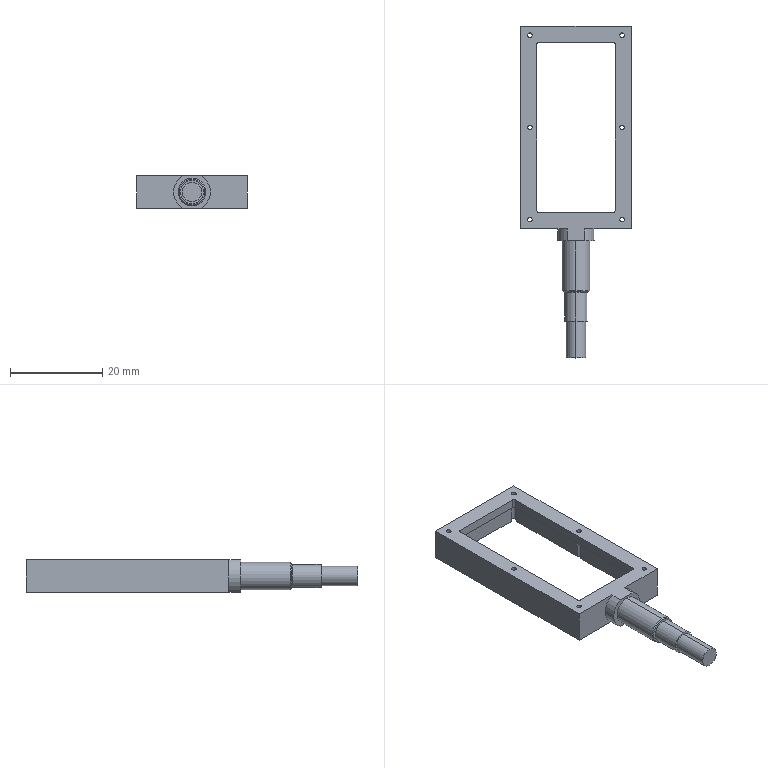NC program | NX | posted with a generic post | part box 24 x 72 x 7 mm
Whole program:
N10 G17 G21 G94 G90
(FLOOR_WALL_1 , TOOL : D10JING)
N12 T11 M6
N14 G54
N16 G17 G0 G90 X11.997 Y52. S9500 M3
N18 G43 Z30. H11
N20 Z-6.
N22 G94 G1 Z-9. F1250.
N24 Y49.
N26 Y-5.
N28 X6.998
N30 Y49.
N32 X6.936 Y51.6
N34 X1.999
N36 Y-5.
N38 X-3.001
N40 Y51.6
N42 X-6.936
N44 X-8. Y49.
N46 Y-5.
N48 Y-8.
N50 Z-6.
N52 G0 Z30.
N54 M5
N56 M2